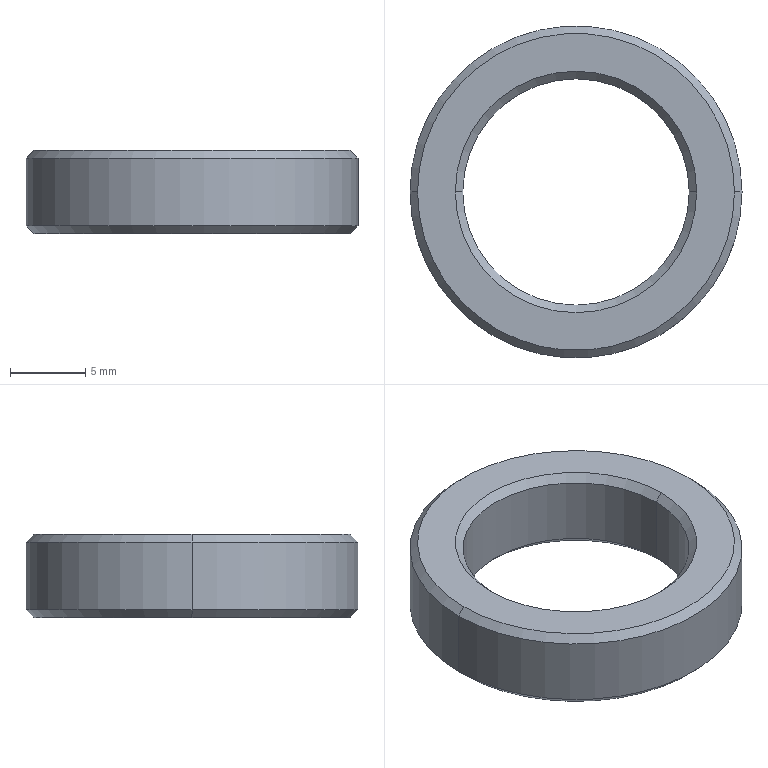Part | SolidWorks | features Chamfer 1, Extrusion 1 | 1 solid | 14 faces | box 22 x 22 x 5.5 mm | volume 1090 mm3 | cone 8 | cylinder 4 | plane 2 | commonest cylinder face diameters 15 x2 22 x2
STEP:
#1=CARTESIAN_POINT('',(-7.5,0.,5.));
#2=VERTEX_POINT('',#1);
#3=CARTESIAN_POINT('',(7.5,0.,5.));
#4=VERTEX_POINT('',#3);
#5=CARTESIAN_POINT('',(0.,0.,5.));
#6=DIRECTION('',(0.,0.,1.));
#7=DIRECTION('',(1.,0.,0.));
#8=AXIS2_PLACEMENT_3D('',#5,#6,#7);
#9=CIRCLE('',#8,7.5);
#10=EDGE_CURVE('',#2,#4,#9,.T.);
#11=ORIENTED_EDGE('',*,*,#10,.F.);
#12=CARTESIAN_POINT('',(-8.,0.,5.5));
#13=VERTEX_POINT('',#12);
#14=CARTESIAN_POINT('',(-7.5,0.,5.));
#15=DIRECTION('',(-0.7071,0.,0.7071));
#16=VECTOR('',#15,1000.);
#17=LINE('',#14,#16);
#18=EDGE_CURVE('',#2,#13,#17,.T.);
#19=ORIENTED_EDGE('',*,*,#18,.T.);
#20=CARTESIAN_POINT('',(8.,0.,5.5));
#21=VERTEX_POINT('',#20);
#22=CARTESIAN_POINT('',(0.,0.,5.5));
#23=DIRECTION('',(0.,0.,-1.));
#24=DIRECTION('',(1.,0.,0.));
#25=AXIS2_PLACEMENT_3D('',#22,#23,#24);
#26=CIRCLE('',#25,8.);
#27=EDGE_CURVE('',#21,#13,#26,.T.);
#28=ORIENTED_EDGE('',*,*,#27,.F.);
#29=CARTESIAN_POINT('',(7.5,0.,5.));
#30=DIRECTION('',(0.7071,0.,0.7071));
#31=VECTOR('',#30,1000.);
#32=LINE('',#29,#31);
#33=EDGE_CURVE('',#4,#21,#32,.T.);
#34=ORIENTED_EDGE('',*,*,#33,.F.);
#35=EDGE_LOOP('',(#11,#19,#28,#34));
#36=FACE_OUTER_BOUND('',#35,.T.);
#37=CARTESIAN_POINT('',(0.,0.,5.));
#38=DIRECTION('',(0.,0.,1.));
#39=DIRECTION('',(1.,0.,0.));
#40=AXIS2_PLACEMENT_3D('',#37,#38,#39);
#41=CONICAL_SURFACE('',#40,7.5,0.7854);
#42=ADVANCED_FACE('',(#36),#41,.F.);
#43=CARTESIAN_POINT('',(7.5,0.,0.5));
#44=VERTEX_POINT('',#43);
#45=CARTESIAN_POINT('',(-7.5,0.,0.5));
#46=VERTEX_POINT('',#45);
#47=CARTESIAN_POINT('',(0.,0.,0.5));
#48=DIRECTION('',(0.,0.,-1.));
#49=DIRECTION('',(1.,0.,0.));
#50=AXIS2_PLACEMENT_3D('',#47,#48,#49);
#51=CIRCLE('',#50,7.5);
#52=EDGE_CURVE('',#44,#46,#51,.T.);
#53=ORIENTED_EDGE('',*,*,#52,.F.);
#54=CARTESIAN_POINT('',(8.,0.,0.));
#55=VERTEX_POINT('',#54);
#56=CARTESIAN_POINT('',(8.,0.,0.));
#57=DIRECTION('',(0.7071,0.,-0.7071));
#58=VECTOR('',#57,1000.);
#59=LINE('',#56,#58);
#60=EDGE_CURVE('',#44,#55,#59,.T.);
#61=ORIENTED_EDGE('',*,*,#60,.T.);
#62=CARTESIAN_POINT('',(-8.,0.,0.));
#63=VERTEX_POINT('',#62);
#64=CARTESIAN_POINT('',(0.,0.,0.));
#65=DIRECTION('',(0.,0.,1.));
#66=DIRECTION('',(1.,0.,0.));
#67=AXIS2_PLACEMENT_3D('',#64,#65,#66);
#68=CIRCLE('',#67,8.);
#69=EDGE_CURVE('',#63,#55,#68,.T.);
#70=ORIENTED_EDGE('',*,*,#69,.F.);
#71=CARTESIAN_POINT('',(-8.,0.,0.));
#72=DIRECTION('',(-0.7071,0.,-0.7071));
#73=VECTOR('',#72,1000.);
#74=LINE('',#71,#73);
#75=EDGE_CURVE('',#46,#63,#74,.T.);
#76=ORIENTED_EDGE('',*,*,#75,.F.);
#77=EDGE_LOOP('',(#53,#61,#70,#76));
#78=FACE_OUTER_BOUND('',#77,.T.);
#79=CARTESIAN_POINT('',(0.,0.,0.));
#80=DIRECTION('',(0.,0.,-1.));
#81=DIRECTION('',(-1.,0.,0.));
#82=AXIS2_PLACEMENT_3D('',#79,#80,#81);
#83=CONICAL_SURFACE('',#82,8.,0.7854);
#84=ADVANCED_FACE('',(#78),#83,.F.);
#85=CARTESIAN_POINT('',(10.5,0.,5.5));
#86=VERTEX_POINT('',#85);
#87=CARTESIAN_POINT('',(-10.5,0.,5.5));
#88=VERTEX_POINT('',#87);
#89=CARTESIAN_POINT('',(0.,0.,5.5));
#90=DIRECTION('',(0.,0.,1.));
#91=DIRECTION('',(1.,0.,0.));
#92=AXIS2_PLACEMENT_3D('',#89,#90,#91);
#93=CIRCLE('',#92,10.5);
#94=EDGE_CURVE('',#86,#88,#93,.T.);
#95=ORIENTED_EDGE('',*,*,#94,.F.);
#96=CARTESIAN_POINT('',(11.,0.,5.));
#97=VERTEX_POINT('',#96);
#98=CARTESIAN_POINT('',(10.5,0.,5.5));
#99=DIRECTION('',(0.7071,0.,-0.7071));
#100=VECTOR('',#99,1000.);
#101=LINE('',#98,#100);
#102=EDGE_CURVE('',#86,#97,#101,.T.);
#103=ORIENTED_EDGE('',*,*,#102,.T.);
#104=CARTESIAN_POINT('',(-11.,0.,5.));
#105=VERTEX_POINT('',#104);
#106=CARTESIAN_POINT('',(0.,0.,5.));
#107=DIRECTION('',(0.,0.,-1.));
#108=DIRECTION('',(1.,0.,0.));
#109=AXIS2_PLACEMENT_3D('',#106,#107,#108);
#110=CIRCLE('',#109,11.);
#111=EDGE_CURVE('',#105,#97,#110,.T.);
#112=ORIENTED_EDGE('',*,*,#111,.F.);
#113=CARTESIAN_POINT('',(-10.5,0.,5.5));
#114=DIRECTION('',(-0.7071,0.,-0.7071));
#115=VECTOR('',#114,1000.);
#116=LINE('',#113,#115);
#117=EDGE_CURVE('',#88,#105,#116,.T.);
#118=ORIENTED_EDGE('',*,*,#117,.F.);
#119=EDGE_LOOP('',(#95,#103,#112,#118));
#120=FACE_OUTER_BOUND('',#119,.T.);
#121=CARTESIAN_POINT('',(0.,0.,5.5));
#122=DIRECTION('',(0.,0.,-1.));
#123=DIRECTION('',(-1.,0.,0.));
#124=AXIS2_PLACEMENT_3D('',#121,#122,#123);
#125=CONICAL_SURFACE('',#124,10.5,0.7854);
#126=ADVANCED_FACE('',(#120),#125,.T.);
#127=CARTESIAN_POINT('',(-10.5,0.,0.));
#128=VERTEX_POINT('',#127);
#129=CARTESIAN_POINT('',(10.5,0.,0.));
#130=VERTEX_POINT('',#129);
#131=CARTESIAN_POINT('',(0.,0.,0.));
#132=DIRECTION('',(0.,0.,-1.));
#133=DIRECTION('',(1.,0.,0.));
#134=AXIS2_PLACEMENT_3D('',#131,#132,#133);
#135=CIRCLE('',#134,10.5);
#136=EDGE_CURVE('',#128,#130,#135,.T.);
#137=ORIENTED_EDGE('',*,*,#136,.F.);
#138=CARTESIAN_POINT('',(-11.,0.,0.5));
#139=VERTEX_POINT('',#138);
#140=CARTESIAN_POINT('',(-11.,0.,0.5));
#141=DIRECTION('',(-0.7071,0.,0.7071));
#142=VECTOR('',#141,1000.);
#143=LINE('',#140,#142);
#144=EDGE_CURVE('',#128,#139,#143,.T.);
#145=ORIENTED_EDGE('',*,*,#144,.T.);
#146=CARTESIAN_POINT('',(11.,0.,0.5));
#147=VERTEX_POINT('',#146);
#148=CARTESIAN_POINT('',(0.,0.,0.5));
#149=DIRECTION('',(0.,0.,1.));
#150=DIRECTION('',(1.,0.,0.));
#151=AXIS2_PLACEMENT_3D('',#148,#149,#150);
#152=CIRCLE('',#151,11.);
#153=EDGE_CURVE('',#147,#139,#152,.T.);
#154=ORIENTED_EDGE('',*,*,#153,.F.);
#155=CARTESIAN_POINT('',(11.,0.,0.5));
#156=DIRECTION('',(0.7071,0.,0.7071));
#157=VECTOR('',#156,1000.);
#158=LINE('',#155,#157);
#159=EDGE_CURVE('',#130,#147,#158,.T.);
#160=ORIENTED_EDGE('',*,*,#159,.F.);
#161=EDGE_LOOP('',(#137,#145,#154,#160));
#162=FACE_OUTER_BOUND('',#161,.T.);
#163=CARTESIAN_POINT('',(0.,0.,0.5));
#164=DIRECTION('',(0.,0.,1.));
#165=DIRECTION('',(1.,0.,0.));
#166=AXIS2_PLACEMENT_3D('',#163,#164,#165);
#167=CONICAL_SURFACE('',#166,11.,0.7854);
#168=ADVANCED_FACE('',(#162),#167,.T.);
#169=ORIENTED_EDGE('',*,*,#10,.T.);
#170=CARTESIAN_POINT('',(7.5,0.,5.5));
#171=DIRECTION('',(0.,0.,-1.));
#172=VECTOR('',#171,1000.);
#173=LINE('',#170,#172);
#174=EDGE_CURVE('',#4,#44,#173,.T.);
#175=ORIENTED_EDGE('',*,*,#174,.T.);
#176=ORIENTED_EDGE('',*,*,#52,.T.);
#177=CARTESIAN_POINT('',(-7.5,0.,5.5));
#178=DIRECTION('',(0.,0.,-1.));
#179=VECTOR('',#178,1000.);
#180=LINE('',#177,#179);
#181=EDGE_CURVE('',#2,#46,#180,.T.);
#182=ORIENTED_EDGE('',*,*,#181,.F.);
#183=EDGE_LOOP('',(#169,#175,#176,#182));
#184=FACE_OUTER_BOUND('',#183,.T.);
#185=CARTESIAN_POINT('',(0.,0.,5.5));
#186=DIRECTION('',(0.,0.,-1.));
#187=DIRECTION('',(-1.,0.,0.));
#188=AXIS2_PLACEMENT_3D('',#185,#186,#187);
#189=CYLINDRICAL_SURFACE('',#188,7.5);
#190=ADVANCED_FACE('',(#184),#189,.F.);
#191=ORIENTED_EDGE('',*,*,#111,.T.);
#192=CARTESIAN_POINT('',(11.,0.,5.5));
#193=DIRECTION('',(0.,0.,-1.));
#194=VECTOR('',#193,1000.);
#195=LINE('',#192,#194);
#196=EDGE_CURVE('',#97,#147,#195,.T.);
#197=ORIENTED_EDGE('',*,*,#196,.T.);
#198=ORIENTED_EDGE('',*,*,#153,.T.);
#199=CARTESIAN_POINT('',(-11.,0.,5.5));
#200=DIRECTION('',(0.,0.,-1.));
#201=VECTOR('',#200,1000.);
#202=LINE('',#199,#201);
#203=EDGE_CURVE('',#105,#139,#202,.T.);
#204=ORIENTED_EDGE('',*,*,#203,.F.);
#205=EDGE_LOOP('',(#191,#197,#198,#204));
#206=FACE_OUTER_BOUND('',#205,.T.);
#207=CARTESIAN_POINT('',(0.,0.,5.5));
#208=DIRECTION('',(0.,0.,-1.));
#209=DIRECTION('',(-1.,0.,0.));
#210=AXIS2_PLACEMENT_3D('',#207,#208,#209);
#211=CYLINDRICAL_SURFACE('',#210,11.);
#212=ADVANCED_FACE('',(#206),#211,.T.);
#213=CARTESIAN_POINT('',(0.,0.,5.5));
#214=DIRECTION('',(0.,0.,1.));
#215=DIRECTION('',(1.,0.,0.));
#216=AXIS2_PLACEMENT_3D('',#213,#214,#215);
#217=CIRCLE('',#216,10.5);
#218=EDGE_CURVE('',#88,#86,#217,.T.);
#219=ORIENTED_EDGE('',*,*,#218,.T.);
#220=ORIENTED_EDGE('',*,*,#94,.T.);
#221=EDGE_LOOP('',(#219,#220));
#222=FACE_OUTER_BOUND('',#221,.T.);
#223=ORIENTED_EDGE('',*,*,#27,.T.);
#224=CARTESIAN_POINT('',(0.,0.,5.5));
#225=DIRECTION('',(0.,0.,-1.));
#226=DIRECTION('',(1.,0.,0.));
#227=AXIS2_PLACEMENT_3D('',#224,#225,#226);
#228=CIRCLE('',#227,8.);
#229=EDGE_CURVE('',#13,#21,#228,.T.);
#230=ORIENTED_EDGE('',*,*,#229,.T.);
#231=EDGE_LOOP('',(#223,#230));
#232=FACE_BOUND('',#231,.T.);
#233=CARTESIAN_POINT('',(0.,0.,5.5));
#234=DIRECTION('',(0.,0.,1.));
#235=DIRECTION('',(1.,0.,0.));
#236=AXIS2_PLACEMENT_3D('',#233,#234,#235);
#237=PLANE('',#236);
#238=ADVANCED_FACE('',(#222,#232),#237,.T.);
#239=CARTESIAN_POINT('',(0.,0.,0.));
#240=DIRECTION('',(0.,0.,-1.));
#241=DIRECTION('',(1.,0.,0.));
#242=AXIS2_PLACEMENT_3D('',#239,#240,#241);
#243=CIRCLE('',#242,10.5);
#244=EDGE_CURVE('',#130,#128,#243,.T.);
#245=ORIENTED_EDGE('',*,*,#244,.T.);
#246=ORIENTED_EDGE('',*,*,#136,.T.);
#247=EDGE_LOOP('',(#245,#246));
#248=FACE_OUTER_BOUND('',#247,.T.);
#249=ORIENTED_EDGE('',*,*,#69,.T.);
#250=CARTESIAN_POINT('',(0.,0.,0.));
#251=DIRECTION('',(0.,0.,1.));
#252=DIRECTION('',(1.,0.,0.));
#253=AXIS2_PLACEMENT_3D('',#250,#251,#252);
#254=CIRCLE('',#253,8.);
#255=EDGE_CURVE('',#55,#63,#254,.T.);
#256=ORIENTED_EDGE('',*,*,#255,.T.);
#257=EDGE_LOOP('',(#249,#256));
#258=FACE_BOUND('',#257,.T.);
#259=CARTESIAN_POINT('',(0.,0.,0.));
#260=DIRECTION('',(0.,0.,1.));
#261=DIRECTION('',(1.,0.,0.));
#262=AXIS2_PLACEMENT_3D('',#259,#260,#261);
#263=PLANE('',#262);
#264=ADVANCED_FACE('',(#248,#258),#263,.F.);
#265=ORIENTED_EDGE('',*,*,#196,.F.);
#266=CARTESIAN_POINT('',(0.,0.,5.));
#267=DIRECTION('',(0.,0.,-1.));
#268=DIRECTION('',(1.,0.,0.));
#269=AXIS2_PLACEMENT_3D('',#266,#267,#268);
#270=CIRCLE('',#269,11.);
#271=EDGE_CURVE('',#97,#105,#270,.T.);
#272=ORIENTED_EDGE('',*,*,#271,.T.);
#273=ORIENTED_EDGE('',*,*,#203,.T.);
#274=CARTESIAN_POINT('',(0.,0.,0.5));
#275=DIRECTION('',(0.,0.,1.));
#276=DIRECTION('',(1.,0.,0.));
#277=AXIS2_PLACEMENT_3D('',#274,#275,#276);
#278=CIRCLE('',#277,11.);
#279=EDGE_CURVE('',#139,#147,#278,.T.);
#280=ORIENTED_EDGE('',*,*,#279,.T.);
#281=EDGE_LOOP('',(#265,#272,#273,#280));
#282=FACE_OUTER_BOUND('',#281,.T.);
#283=CARTESIAN_POINT('',(0.,0.,5.5));
#284=DIRECTION('',(0.,0.,-1.));
#285=DIRECTION('',(-1.,0.,0.));
#286=AXIS2_PLACEMENT_3D('',#283,#284,#285);
#287=CYLINDRICAL_SURFACE('',#286,11.);
#288=ADVANCED_FACE('',(#282),#287,.T.);
#289=ORIENTED_EDGE('',*,*,#174,.F.);
#290=CARTESIAN_POINT('',(0.,0.,5.));
#291=DIRECTION('',(0.,0.,1.));
#292=DIRECTION('',(1.,0.,0.));
#293=AXIS2_PLACEMENT_3D('',#290,#291,#292);
#294=CIRCLE('',#293,7.5);
#295=EDGE_CURVE('',#4,#2,#294,.T.);
#296=ORIENTED_EDGE('',*,*,#295,.T.);
#297=ORIENTED_EDGE('',*,*,#181,.T.);
#298=CARTESIAN_POINT('',(0.,0.,0.5));
#299=DIRECTION('',(0.,0.,-1.));
#300=DIRECTION('',(1.,0.,0.));
#301=AXIS2_PLACEMENT_3D('',#298,#299,#300);
#302=CIRCLE('',#301,7.5);
#303=EDGE_CURVE('',#46,#44,#302,.T.);
#304=ORIENTED_EDGE('',*,*,#303,.T.);
#305=EDGE_LOOP('',(#289,#296,#297,#304));
#306=FACE_OUTER_BOUND('',#305,.T.);
#307=CARTESIAN_POINT('',(0.,0.,5.5));
#308=DIRECTION('',(0.,0.,-1.));
#309=DIRECTION('',(-1.,0.,0.));
#310=AXIS2_PLACEMENT_3D('',#307,#308,#309);
#311=CYLINDRICAL_SURFACE('',#310,7.5);
#312=ADVANCED_FACE('',(#306),#311,.F.);
#313=ORIENTED_EDGE('',*,*,#144,.F.);
#314=ORIENTED_EDGE('',*,*,#244,.F.);
#315=ORIENTED_EDGE('',*,*,#159,.T.);
#316=ORIENTED_EDGE('',*,*,#279,.F.);
#317=EDGE_LOOP('',(#313,#314,#315,#316));
#318=FACE_OUTER_BOUND('',#317,.T.);
#319=CARTESIAN_POINT('',(0.,0.,0.5));
#320=DIRECTION('',(0.,0.,1.));
#321=DIRECTION('',(1.,0.,0.));
#322=AXIS2_PLACEMENT_3D('',#319,#320,#321);
#323=CONICAL_SURFACE('',#322,11.,0.7854);
#324=ADVANCED_FACE('',(#318),#323,.T.);
#325=ORIENTED_EDGE('',*,*,#102,.F.);
#326=ORIENTED_EDGE('',*,*,#218,.F.);
#327=ORIENTED_EDGE('',*,*,#117,.T.);
#328=ORIENTED_EDGE('',*,*,#271,.F.);
#329=EDGE_LOOP('',(#325,#326,#327,#328));
#330=FACE_OUTER_BOUND('',#329,.T.);
#331=CARTESIAN_POINT('',(0.,0.,5.5));
#332=DIRECTION('',(0.,0.,-1.));
#333=DIRECTION('',(-1.,0.,0.));
#334=AXIS2_PLACEMENT_3D('',#331,#332,#333);
#335=CONICAL_SURFACE('',#334,10.5,0.7854);
#336=ADVANCED_FACE('',(#330),#335,.T.);
#337=ORIENTED_EDGE('',*,*,#60,.F.);
#338=ORIENTED_EDGE('',*,*,#303,.F.);
#339=ORIENTED_EDGE('',*,*,#75,.T.);
#340=ORIENTED_EDGE('',*,*,#255,.F.);
#341=EDGE_LOOP('',(#337,#338,#339,#340));
#342=FACE_OUTER_BOUND('',#341,.T.);
#343=CARTESIAN_POINT('',(0.,0.,0.));
#344=DIRECTION('',(0.,0.,-1.));
#345=DIRECTION('',(-1.,0.,0.));
#346=AXIS2_PLACEMENT_3D('',#343,#344,#345);
#347=CONICAL_SURFACE('',#346,8.,0.7854);
#348=ADVANCED_FACE('',(#342),#347,.F.);
#349=ORIENTED_EDGE('',*,*,#18,.F.);
#350=ORIENTED_EDGE('',*,*,#295,.F.);
#351=ORIENTED_EDGE('',*,*,#33,.T.);
#352=ORIENTED_EDGE('',*,*,#229,.F.);
#353=EDGE_LOOP('',(#349,#350,#351,#352));
#354=FACE_OUTER_BOUND('',#353,.T.);
#355=CARTESIAN_POINT('',(0.,0.,5.));
#356=DIRECTION('',(0.,0.,1.));
#357=DIRECTION('',(1.,0.,0.));
#358=AXIS2_PLACEMENT_3D('',#355,#356,#357);
#359=CONICAL_SURFACE('',#358,7.5,0.7854);
#360=ADVANCED_FACE('',(#354),#359,.F.);
#361=CLOSED_SHELL('',(#42,#84,#126,#168,#190,#212,#238,#264,#288,#312,#324,#336,#348,#360));
#362=MANIFOLD_SOLID_BREP('',#361);
#363=CARTESIAN_POINT('',(0.,0.,0.));
#364=DIRECTION('',(0.,0.,1.));
#365=DIRECTION('',(1.,0.,0.));
#366=AXIS2_PLACEMENT_3D('',#363,#364,#365);
#367=(LENGTH_UNIT()NAMED_UNIT(*)SI_UNIT(.MILLI.,.METRE.));
#368=UNCERTAINTY_MEASURE_WITH_UNIT(LENGTH_MEASURE(0.00001),#367,'','');
#369=(NAMED_UNIT(*)PLANE_ANGLE_UNIT()SI_UNIT($,.RADIAN.));
#370=(NAMED_UNIT(*)SI_UNIT($,.STERADIAN.)SOLID_ANGLE_UNIT());
#371=(GEOMETRIC_REPRESENTATION_CONTEXT(3)GLOBAL_UNCERTAINTY_ASSIGNED_CONTEXT((#368))GLOBAL_UNIT_ASSIGNED_CONTEXT((#367,#369,#370))REPRESENTATION_CONTEXT('',''));
#372=ADVANCED_BREP_SHAPE_REPRESENTATION('',(#362,#366),#371);